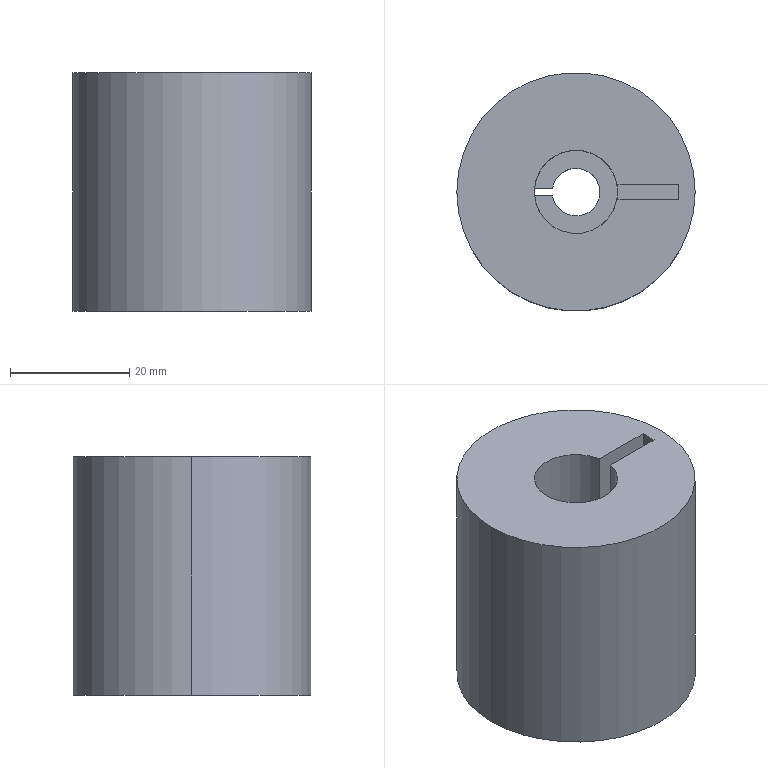Part | SolidWorks | features ICE 4, Extrusion 1 | 1 solid | 17 faces | box 40 x 40 x 40 mm | volume 44793 mm3 | plane 11 | cylinder 6 | commonest cylinder face diameters 8 x2 14 x2 40 x2
STEP:
#1=CARTESIAN_POINT('',(-7.,0.,13.));
#2=VERTEX_POINT('',#1);
#3=CARTESIAN_POINT('',(-6.971,-0.64,13.));
#4=VERTEX_POINT('',#3);
#5=CARTESIAN_POINT('',(0.,0.,13.));
#6=DIRECTION('',(0.,0.,1.));
#7=DIRECTION('',(-1.,0.,0.));
#8=AXIS2_PLACEMENT_3D('',#5,#6,#7);
#9=CIRCLE('',#8,7.);
#10=EDGE_CURVE('',#2,#4,#9,.T.);
#11=ORIENTED_EDGE('',*,*,#10,.F.);
#12=CARTESIAN_POINT('',(-7.,0.,40.));
#13=VERTEX_POINT('',#12);
#14=CARTESIAN_POINT('',(-7.,0.,12.));
#15=DIRECTION('',(0.,0.,1.));
#16=VECTOR('',#15,1000.);
#17=LINE('',#14,#16);
#18=EDGE_CURVE('',#2,#13,#17,.T.);
#19=ORIENTED_EDGE('',*,*,#18,.T.);
#20=CARTESIAN_POINT('',(6.878,-1.3,40.));
#21=VERTEX_POINT('',#20);
#22=CARTESIAN_POINT('',(0.,0.,40.));
#23=DIRECTION('',(0.,0.,1.));
#24=DIRECTION('',(1.,0.,0.));
#25=AXIS2_PLACEMENT_3D('',#22,#23,#24);
#26=CIRCLE('',#25,7.);
#27=EDGE_CURVE('',#13,#21,#26,.T.);
#28=ORIENTED_EDGE('',*,*,#27,.T.);
#29=CARTESIAN_POINT('',(6.878,-1.3,27.));
#30=VERTEX_POINT('',#29);
#31=CARTESIAN_POINT('',(6.878,-1.3,27.));
#32=DIRECTION('',(0.,0.,1.));
#33=VECTOR('',#32,1000.);
#34=LINE('',#31,#33);
#35=EDGE_CURVE('',#30,#21,#34,.T.);
#36=ORIENTED_EDGE('',*,*,#35,.F.);
#37=CARTESIAN_POINT('',(7.,0.,27.));
#38=VERTEX_POINT('',#37);
#39=CARTESIAN_POINT('',(0.,0.,27.));
#40=DIRECTION('',(0.,0.,-1.));
#41=DIRECTION('',(1.,0.,0.));
#42=AXIS2_PLACEMENT_3D('',#39,#40,#41);
#43=CIRCLE('',#42,7.);
#44=EDGE_CURVE('',#38,#30,#43,.T.);
#45=ORIENTED_EDGE('',*,*,#44,.F.);
#46=CARTESIAN_POINT('',(7.,0.,12.));
#47=VERTEX_POINT('',#46);
#48=CARTESIAN_POINT('',(7.,0.,12.));
#49=DIRECTION('',(0.,0.,1.));
#50=VECTOR('',#49,1000.);
#51=LINE('',#48,#50);
#52=EDGE_CURVE('',#47,#38,#51,.T.);
#53=ORIENTED_EDGE('',*,*,#52,.F.);
#54=CARTESIAN_POINT('',(-6.971,-0.64,12.));
#55=VERTEX_POINT('',#54);
#56=CARTESIAN_POINT('',(0.,0.,12.));
#57=DIRECTION('',(0.,0.,1.));
#58=DIRECTION('',(1.,0.,0.));
#59=AXIS2_PLACEMENT_3D('',#56,#57,#58);
#60=CIRCLE('',#59,7.);
#61=EDGE_CURVE('',#55,#47,#60,.T.);
#62=ORIENTED_EDGE('',*,*,#61,.F.);
#63=CARTESIAN_POINT('',(-6.971,-0.64,12.));
#64=DIRECTION('',(0.,0.,1.));
#65=VECTOR('',#64,1000.);
#66=LINE('',#63,#65);
#67=EDGE_CURVE('',#55,#4,#66,.T.);
#68=ORIENTED_EDGE('',*,*,#67,.T.);
#69=EDGE_LOOP('',(#11,#19,#28,#36,#45,#53,#62,#68));
#70=FACE_OUTER_BOUND('',#69,.T.);
#71=CARTESIAN_POINT('',(0.,0.,12.));
#72=DIRECTION('',(0.,0.,1.));
#73=DIRECTION('',(1.,0.,0.));
#74=AXIS2_PLACEMENT_3D('',#71,#72,#73);
#75=CYLINDRICAL_SURFACE('',#74,7.);
#76=ADVANCED_FACE('',(#70),#75,.F.);
#77=CARTESIAN_POINT('',(20.,0.,40.));
#78=VERTEX_POINT('',#77);
#79=CARTESIAN_POINT('',(-20.,0.,40.));
#80=VERTEX_POINT('',#79);
#81=CARTESIAN_POINT('',(0.,0.,40.));
#82=DIRECTION('',(0.,0.,1.));
#83=DIRECTION('',(1.,0.,0.));
#84=AXIS2_PLACEMENT_3D('',#81,#82,#83);
#85=CIRCLE('',#84,20.);
#86=EDGE_CURVE('',#78,#80,#85,.T.);
#87=ORIENTED_EDGE('',*,*,#86,.F.);
#88=CARTESIAN_POINT('',(20.,0.,0.));
#89=VERTEX_POINT('',#88);
#90=CARTESIAN_POINT('',(20.,0.,40.));
#91=DIRECTION('',(0.,0.,-1.));
#92=VECTOR('',#91,1000.);
#93=LINE('',#90,#92);
#94=EDGE_CURVE('',#78,#89,#93,.T.);
#95=ORIENTED_EDGE('',*,*,#94,.T.);
#96=CARTESIAN_POINT('',(-20.,0.,0.));
#97=VERTEX_POINT('',#96);
#98=CARTESIAN_POINT('',(0.,0.,0.));
#99=DIRECTION('',(0.,0.,1.));
#100=DIRECTION('',(1.,0.,0.));
#101=AXIS2_PLACEMENT_3D('',#98,#99,#100);
#102=CIRCLE('',#101,20.);
#103=EDGE_CURVE('',#89,#97,#102,.T.);
#104=ORIENTED_EDGE('',*,*,#103,.T.);
#105=CARTESIAN_POINT('',(-20.,0.,40.));
#106=DIRECTION('',(0.,0.,-1.));
#107=VECTOR('',#106,1000.);
#108=LINE('',#105,#107);
#109=EDGE_CURVE('',#80,#97,#108,.T.);
#110=ORIENTED_EDGE('',*,*,#109,.F.);
#111=EDGE_LOOP('',(#87,#95,#104,#110));
#112=FACE_OUTER_BOUND('',#111,.T.);
#113=CARTESIAN_POINT('',(0.,0.,40.));
#114=DIRECTION('',(0.,0.,-1.));
#115=DIRECTION('',(-1.,0.,0.));
#116=AXIS2_PLACEMENT_3D('',#113,#114,#115);
#117=CYLINDRICAL_SURFACE('',#116,20.);
#118=ADVANCED_FACE('',(#112),#117,.T.);
#119=CARTESIAN_POINT('',(4.,0.,0.));
#120=VERTEX_POINT('',#119);
#121=CARTESIAN_POINT('',(-3.948,0.64,0.));
#122=VERTEX_POINT('',#121);
#123=CARTESIAN_POINT('',(0.,0.,0.));
#124=DIRECTION('',(0.,0.,1.));
#125=DIRECTION('',(1.,0.,0.));
#126=AXIS2_PLACEMENT_3D('',#123,#124,#125);
#127=CIRCLE('',#126,4.);
#128=EDGE_CURVE('',#120,#122,#127,.T.);
#129=ORIENTED_EDGE('',*,*,#128,.F.);
#130=CARTESIAN_POINT('',(4.,0.,12.));
#131=VERTEX_POINT('',#130);
#132=CARTESIAN_POINT('',(4.,0.,0.));
#133=DIRECTION('',(0.,0.,1.));
#134=VECTOR('',#133,1000.);
#135=LINE('',#132,#134);
#136=EDGE_CURVE('',#120,#131,#135,.T.);
#137=ORIENTED_EDGE('',*,*,#136,.T.);
#138=CARTESIAN_POINT('',(-3.948,0.64,12.));
#139=VERTEX_POINT('',#138);
#140=CARTESIAN_POINT('',(0.,0.,12.));
#141=DIRECTION('',(0.,0.,-1.));
#142=DIRECTION('',(1.,0.,0.));
#143=AXIS2_PLACEMENT_3D('',#140,#141,#142);
#144=CIRCLE('',#143,4.);
#145=EDGE_CURVE('',#139,#131,#144,.T.);
#146=ORIENTED_EDGE('',*,*,#145,.F.);
#147=CARTESIAN_POINT('',(-3.948,0.64,13.));
#148=DIRECTION('',(0.,0.,-1.));
#149=VECTOR('',#148,1000.);
#150=LINE('',#147,#149);
#151=EDGE_CURVE('',#139,#122,#150,.T.);
#152=ORIENTED_EDGE('',*,*,#151,.T.);
#153=EDGE_LOOP('',(#129,#137,#146,#152));
#154=FACE_OUTER_BOUND('',#153,.T.);
#155=CARTESIAN_POINT('',(0.,0.,0.));
#156=DIRECTION('',(0.,0.,1.));
#157=DIRECTION('',(1.,0.,0.));
#158=AXIS2_PLACEMENT_3D('',#155,#156,#157);
#159=CYLINDRICAL_SURFACE('',#158,4.);
#160=ADVANCED_FACE('',(#154),#159,.F.);
#161=ORIENTED_EDGE('',*,*,#136,.F.);
#162=CARTESIAN_POINT('',(-3.948,-0.64,0.));
#163=VERTEX_POINT('',#162);
#164=CARTESIAN_POINT('',(0.,0.,0.));
#165=DIRECTION('',(0.,0.,1.));
#166=DIRECTION('',(1.,0.,0.));
#167=AXIS2_PLACEMENT_3D('',#164,#165,#166);
#168=CIRCLE('',#167,4.);
#169=EDGE_CURVE('',#163,#120,#168,.T.);
#170=ORIENTED_EDGE('',*,*,#169,.F.);
#171=CARTESIAN_POINT('',(-3.948,-0.64,12.));
#172=VERTEX_POINT('',#171);
#173=CARTESIAN_POINT('',(-3.948,-0.64,13.));
#174=DIRECTION('',(0.,0.,-1.));
#175=VECTOR('',#174,1000.);
#176=LINE('',#173,#175);
#177=EDGE_CURVE('',#172,#163,#176,.T.);
#178=ORIENTED_EDGE('',*,*,#177,.F.);
#179=CARTESIAN_POINT('',(0.,0.,12.));
#180=DIRECTION('',(0.,0.,-1.));
#181=DIRECTION('',(1.,0.,0.));
#182=AXIS2_PLACEMENT_3D('',#179,#180,#181);
#183=CIRCLE('',#182,4.);
#184=EDGE_CURVE('',#131,#172,#183,.T.);
#185=ORIENTED_EDGE('',*,*,#184,.F.);
#186=EDGE_LOOP('',(#161,#170,#178,#185));
#187=FACE_OUTER_BOUND('',#186,.T.);
#188=CARTESIAN_POINT('',(0.,0.,0.));
#189=DIRECTION('',(0.,0.,1.));
#190=DIRECTION('',(1.,0.,0.));
#191=AXIS2_PLACEMENT_3D('',#188,#189,#190);
#192=CYLINDRICAL_SURFACE('',#191,4.);
#193=ADVANCED_FACE('',(#187),#192,.F.);
#194=ORIENTED_EDGE('',*,*,#94,.F.);
#195=CARTESIAN_POINT('',(0.,0.,40.));
#196=DIRECTION('',(0.,0.,1.));
#197=DIRECTION('',(1.,0.,0.));
#198=AXIS2_PLACEMENT_3D('',#195,#196,#197);
#199=CIRCLE('',#198,20.);
#200=EDGE_CURVE('',#80,#78,#199,.T.);
#201=ORIENTED_EDGE('',*,*,#200,.F.);
#202=ORIENTED_EDGE('',*,*,#109,.T.);
#203=CARTESIAN_POINT('',(0.,0.,0.));
#204=DIRECTION('',(0.,0.,1.));
#205=DIRECTION('',(1.,0.,0.));
#206=AXIS2_PLACEMENT_3D('',#203,#204,#205);
#207=CIRCLE('',#206,20.);
#208=EDGE_CURVE('',#97,#89,#207,.T.);
#209=ORIENTED_EDGE('',*,*,#208,.T.);
#210=EDGE_LOOP('',(#194,#201,#202,#209));
#211=FACE_OUTER_BOUND('',#210,.T.);
#212=CARTESIAN_POINT('',(0.,0.,40.));
#213=DIRECTION('',(0.,0.,-1.));
#214=DIRECTION('',(-1.,0.,0.));
#215=AXIS2_PLACEMENT_3D('',#212,#213,#214);
#216=CYLINDRICAL_SURFACE('',#215,20.);
#217=ADVANCED_FACE('',(#211),#216,.T.);
#218=CARTESIAN_POINT('',(17.228,1.3,40.));
#219=VERTEX_POINT('',#218);
#220=CARTESIAN_POINT('',(6.878,1.3,40.));
#221=VERTEX_POINT('',#220);
#222=CARTESIAN_POINT('',(17.228,1.3,40.));
#223=DIRECTION('',(-1.,0.,0.));
#224=VECTOR('',#223,1000.);
#225=LINE('',#222,#224);
#226=EDGE_CURVE('',#219,#221,#225,.T.);
#227=ORIENTED_EDGE('',*,*,#226,.F.);
#228=CARTESIAN_POINT('',(17.228,-1.3,40.));
#229=VERTEX_POINT('',#228);
#230=CARTESIAN_POINT('',(17.228,-1.3,40.));
#231=DIRECTION('',(0.,1.,0.));
#232=VECTOR('',#231,1000.);
#233=LINE('',#230,#232);
#234=EDGE_CURVE('',#229,#219,#233,.T.);
#235=ORIENTED_EDGE('',*,*,#234,.F.);
#236=CARTESIAN_POINT('',(17.228,-1.3,40.));
#237=DIRECTION('',(1.,0.,0.));
#238=VECTOR('',#237,1000.);
#239=LINE('',#236,#238);
#240=EDGE_CURVE('',#21,#229,#239,.T.);
#241=ORIENTED_EDGE('',*,*,#240,.F.);
#242=ORIENTED_EDGE('',*,*,#27,.F.);
#243=CARTESIAN_POINT('',(0.,0.,40.));
#244=DIRECTION('',(0.,0.,1.));
#245=DIRECTION('',(1.,0.,0.));
#246=AXIS2_PLACEMENT_3D('',#243,#244,#245);
#247=CIRCLE('',#246,7.);
#248=EDGE_CURVE('',#221,#13,#247,.T.);
#249=ORIENTED_EDGE('',*,*,#248,.F.);
#250=EDGE_LOOP('',(#227,#235,#241,#242,#249));
#251=FACE_BOUND('',#250,.T.);
#252=ORIENTED_EDGE('',*,*,#200,.T.);
#253=ORIENTED_EDGE('',*,*,#86,.T.);
#254=EDGE_LOOP('',(#252,#253));
#255=FACE_OUTER_BOUND('',#254,.T.);
#256=CARTESIAN_POINT('',(0.,0.,40.));
#257=DIRECTION('',(0.,0.,1.));
#258=DIRECTION('',(1.,0.,0.));
#259=AXIS2_PLACEMENT_3D('',#256,#257,#258);
#260=PLANE('',#259);
#261=ADVANCED_FACE('',(#251,#255),#260,.T.);
#262=ORIENTED_EDGE('',*,*,#169,.T.);
#263=ORIENTED_EDGE('',*,*,#128,.T.);
#264=CARTESIAN_POINT('',(-16.948,0.64,0.));
#265=VERTEX_POINT('',#264);
#266=CARTESIAN_POINT('',(-16.948,0.64,0.));
#267=DIRECTION('',(1.,0.,0.));
#268=VECTOR('',#267,1000.);
#269=LINE('',#266,#268);
#270=EDGE_CURVE('',#265,#122,#269,.T.);
#271=ORIENTED_EDGE('',*,*,#270,.F.);
#272=CARTESIAN_POINT('',(-16.948,-0.64,0.));
#273=VERTEX_POINT('',#272);
#274=CARTESIAN_POINT('',(-16.948,-0.64,0.));
#275=DIRECTION('',(0.,1.,0.));
#276=VECTOR('',#275,1000.);
#277=LINE('',#274,#276);
#278=EDGE_CURVE('',#273,#265,#277,.T.);
#279=ORIENTED_EDGE('',*,*,#278,.F.);
#280=CARTESIAN_POINT('',(-16.948,-0.64,0.));
#281=DIRECTION('',(-1.,0.,0.));
#282=VECTOR('',#281,1000.);
#283=LINE('',#280,#282);
#284=EDGE_CURVE('',#163,#273,#283,.T.);
#285=ORIENTED_EDGE('',*,*,#284,.F.);
#286=EDGE_LOOP('',(#262,#263,#271,#279,#285));
#287=FACE_BOUND('',#286,.T.);
#288=ORIENTED_EDGE('',*,*,#208,.F.);
#289=ORIENTED_EDGE('',*,*,#103,.F.);
#290=EDGE_LOOP('',(#288,#289));
#291=FACE_OUTER_BOUND('',#290,.T.);
#292=CARTESIAN_POINT('',(0.,0.,0.));
#293=DIRECTION('',(0.,0.,1.));
#294=DIRECTION('',(1.,0.,0.));
#295=AXIS2_PLACEMENT_3D('',#292,#293,#294);
#296=PLANE('',#295);
#297=ADVANCED_FACE('',(#287,#291),#296,.F.);
#298=CARTESIAN_POINT('',(-6.971,0.64,12.));
#299=VERTEX_POINT('',#298);
#300=CARTESIAN_POINT('',(0.,0.64,12.));
#301=DIRECTION('',(-1.,0.,0.));
#302=VECTOR('',#301,1000.);
#303=LINE('',#300,#302);
#304=EDGE_CURVE('',#139,#299,#303,.T.);
#305=ORIENTED_EDGE('',*,*,#304,.F.);
#306=ORIENTED_EDGE('',*,*,#145,.T.);
#307=ORIENTED_EDGE('',*,*,#184,.T.);
#308=CARTESIAN_POINT('',(0.,-0.64,12.));
#309=DIRECTION('',(1.,0.,0.));
#310=VECTOR('',#309,1000.);
#311=LINE('',#308,#310);
#312=EDGE_CURVE('',#55,#172,#311,.T.);
#313=ORIENTED_EDGE('',*,*,#312,.F.);
#314=ORIENTED_EDGE('',*,*,#61,.T.);
#315=CARTESIAN_POINT('',(0.,0.,12.));
#316=DIRECTION('',(0.,0.,1.));
#317=DIRECTION('',(1.,0.,0.));
#318=AXIS2_PLACEMENT_3D('',#315,#316,#317);
#319=CIRCLE('',#318,7.);
#320=EDGE_CURVE('',#47,#299,#319,.T.);
#321=ORIENTED_EDGE('',*,*,#320,.T.);
#322=EDGE_LOOP('',(#305,#306,#307,#313,#314,#321));
#323=FACE_OUTER_BOUND('',#322,.T.);
#324=CARTESIAN_POINT('',(0.,0.,12.));
#325=DIRECTION('',(0.,0.,1.));
#326=DIRECTION('',(1.,0.,0.));
#327=AXIS2_PLACEMENT_3D('',#324,#325,#326);
#328=PLANE('',#327);
#329=ADVANCED_FACE('',(#323),#328,.T.);
#330=ORIENTED_EDGE('',*,*,#18,.F.);
#331=CARTESIAN_POINT('',(-6.971,0.64,13.));
#332=VERTEX_POINT('',#331);
#333=CARTESIAN_POINT('',(0.,0.,13.));
#334=DIRECTION('',(0.,0.,1.));
#335=DIRECTION('',(-1.,0.,0.));
#336=AXIS2_PLACEMENT_3D('',#333,#334,#335);
#337=CIRCLE('',#336,7.);
#338=EDGE_CURVE('',#332,#2,#337,.T.);
#339=ORIENTED_EDGE('',*,*,#338,.F.);
#340=CARTESIAN_POINT('',(-6.971,0.64,12.));
#341=DIRECTION('',(0.,0.,-1.));
#342=VECTOR('',#341,1000.);
#343=LINE('',#340,#342);
#344=EDGE_CURVE('',#332,#299,#343,.T.);
#345=ORIENTED_EDGE('',*,*,#344,.T.);
#346=ORIENTED_EDGE('',*,*,#320,.F.);
#347=ORIENTED_EDGE('',*,*,#52,.T.);
#348=CARTESIAN_POINT('',(6.878,1.3,27.));
#349=VERTEX_POINT('',#348);
#350=CARTESIAN_POINT('',(0.,0.,27.));
#351=DIRECTION('',(0.,0.,-1.));
#352=DIRECTION('',(1.,0.,0.));
#353=AXIS2_PLACEMENT_3D('',#350,#351,#352);
#354=CIRCLE('',#353,7.);
#355=EDGE_CURVE('',#349,#38,#354,.T.);
#356=ORIENTED_EDGE('',*,*,#355,.F.);
#357=CARTESIAN_POINT('',(6.878,1.3,27.));
#358=DIRECTION('',(0.,0.,1.));
#359=VECTOR('',#358,1000.);
#360=LINE('',#357,#359);
#361=EDGE_CURVE('',#349,#221,#360,.T.);
#362=ORIENTED_EDGE('',*,*,#361,.T.);
#363=ORIENTED_EDGE('',*,*,#248,.T.);
#364=EDGE_LOOP('',(#330,#339,#345,#346,#347,#356,#362,#363));
#365=FACE_OUTER_BOUND('',#364,.T.);
#366=CARTESIAN_POINT('',(0.,0.,12.));
#367=DIRECTION('',(0.,0.,1.));
#368=DIRECTION('',(1.,0.,0.));
#369=AXIS2_PLACEMENT_3D('',#366,#367,#368);
#370=CYLINDRICAL_SURFACE('',#369,7.);
#371=ADVANCED_FACE('',(#365),#370,.F.);
#372=ORIENTED_EDGE('',*,*,#226,.T.);
#373=ORIENTED_EDGE('',*,*,#361,.F.);
#374=CARTESIAN_POINT('',(17.228,1.3,27.));
#375=VERTEX_POINT('',#374);
#376=CARTESIAN_POINT('',(17.228,1.3,27.));
#377=DIRECTION('',(-1.,0.,0.));
#378=VECTOR('',#377,1000.);
#379=LINE('',#376,#378);
#380=EDGE_CURVE('',#375,#349,#379,.T.);
#381=ORIENTED_EDGE('',*,*,#380,.F.);
#382=CARTESIAN_POINT('',(17.228,1.3,27.));
#383=DIRECTION('',(0.,0.,1.));
#384=VECTOR('',#383,1000.);
#385=LINE('',#382,#384);
#386=EDGE_CURVE('',#375,#219,#385,.T.);
#387=ORIENTED_EDGE('',*,*,#386,.T.);
#388=EDGE_LOOP('',(#372,#373,#381,#387));
#389=FACE_OUTER_BOUND('',#388,.T.);
#390=CARTESIAN_POINT('',(17.228,1.3,27.));
#391=DIRECTION('',(0.,1.,0.));
#392=DIRECTION('',(-1.,0.,0.));
#393=AXIS2_PLACEMENT_3D('',#390,#391,#392);
#394=PLANE('',#393);
#395=ADVANCED_FACE('',(#389),#394,.F.);
#396=ORIENTED_EDGE('',*,*,#234,.T.);
#397=ORIENTED_EDGE('',*,*,#386,.F.);
#398=CARTESIAN_POINT('',(17.228,-1.3,27.));
#399=VERTEX_POINT('',#398);
#400=CARTESIAN_POINT('',(17.228,-1.3,27.));
#401=DIRECTION('',(0.,1.,0.));
#402=VECTOR('',#401,1000.);
#403=LINE('',#400,#402);
#404=EDGE_CURVE('',#399,#375,#403,.T.);
#405=ORIENTED_EDGE('',*,*,#404,.F.);
#406=CARTESIAN_POINT('',(17.228,-1.3,27.));
#407=DIRECTION('',(0.,0.,1.));
#408=VECTOR('',#407,1000.);
#409=LINE('',#406,#408);
#410=EDGE_CURVE('',#399,#229,#409,.T.);
#411=ORIENTED_EDGE('',*,*,#410,.T.);
#412=EDGE_LOOP('',(#396,#397,#405,#411));
#413=FACE_OUTER_BOUND('',#412,.T.);
#414=CARTESIAN_POINT('',(17.228,-1.3,27.));
#415=DIRECTION('',(1.,0.,0.));
#416=DIRECTION('',(0.,0.,-1.));
#417=AXIS2_PLACEMENT_3D('',#414,#415,#416);
#418=PLANE('',#417);
#419=ADVANCED_FACE('',(#413),#418,.F.);
#420=ORIENTED_EDGE('',*,*,#240,.T.);
#421=ORIENTED_EDGE('',*,*,#410,.F.);
#422=CARTESIAN_POINT('',(17.228,-1.3,27.));
#423=DIRECTION('',(1.,0.,0.));
#424=VECTOR('',#423,1000.);
#425=LINE('',#422,#424);
#426=EDGE_CURVE('',#30,#399,#425,.T.);
#427=ORIENTED_EDGE('',*,*,#426,.F.);
#428=ORIENTED_EDGE('',*,*,#35,.T.);
#429=EDGE_LOOP('',(#420,#421,#427,#428));
#430=FACE_OUTER_BOUND('',#429,.T.);
#431=CARTESIAN_POINT('',(17.228,-1.3,27.));
#432=DIRECTION('',(0.,-1.,0.));
#433=DIRECTION('',(1.,0.,0.));
#434=AXIS2_PLACEMENT_3D('',#431,#432,#433);
#435=PLANE('',#434);
#436=ADVANCED_FACE('',(#430),#435,.F.);
#437=ORIENTED_EDGE('',*,*,#355,.T.);
#438=ORIENTED_EDGE('',*,*,#44,.T.);
#439=ORIENTED_EDGE('',*,*,#426,.T.);
#440=ORIENTED_EDGE('',*,*,#404,.T.);
#441=ORIENTED_EDGE('',*,*,#380,.T.);
#442=EDGE_LOOP('',(#437,#438,#439,#440,#441));
#443=FACE_OUTER_BOUND('',#442,.T.);
#444=CARTESIAN_POINT('',(0.,0.,27.));
#445=DIRECTION('',(0.,0.,1.));
#446=DIRECTION('',(1.,0.,0.));
#447=AXIS2_PLACEMENT_3D('',#444,#445,#446);
#448=PLANE('',#447);
#449=ADVANCED_FACE('',(#443),#448,.T.);
#450=ORIENTED_EDGE('',*,*,#338,.T.);
#451=ORIENTED_EDGE('',*,*,#10,.T.);
#452=CARTESIAN_POINT('',(-16.948,-0.64,13.));
#453=VERTEX_POINT('',#452);
#454=CARTESIAN_POINT('',(-16.948,-0.64,13.));
#455=DIRECTION('',(-1.,0.,0.));
#456=VECTOR('',#455,1000.);
#457=LINE('',#454,#456);
#458=EDGE_CURVE('',#4,#453,#457,.T.);
#459=ORIENTED_EDGE('',*,*,#458,.T.);
#460=CARTESIAN_POINT('',(-16.948,0.64,13.));
#461=VERTEX_POINT('',#460);
#462=CARTESIAN_POINT('',(-16.948,-0.64,13.));
#463=DIRECTION('',(0.,1.,0.));
#464=VECTOR('',#463,1000.);
#465=LINE('',#462,#464);
#466=EDGE_CURVE('',#453,#461,#465,.T.);
#467=ORIENTED_EDGE('',*,*,#466,.T.);
#468=CARTESIAN_POINT('',(-16.948,0.64,13.));
#469=DIRECTION('',(1.,0.,0.));
#470=VECTOR('',#469,1000.);
#471=LINE('',#468,#470);
#472=EDGE_CURVE('',#461,#332,#471,.T.);
#473=ORIENTED_EDGE('',*,*,#472,.T.);
#474=EDGE_LOOP('',(#450,#451,#459,#467,#473));
#475=FACE_OUTER_BOUND('',#474,.T.);
#476=CARTESIAN_POINT('',(0.,0.,13.));
#477=DIRECTION('',(0.,0.,-1.));
#478=DIRECTION('',(-1.,0.,0.));
#479=AXIS2_PLACEMENT_3D('',#476,#477,#478);
#480=PLANE('',#479);
#481=ADVANCED_FACE('',(#475),#480,.T.);
#482=ORIENTED_EDGE('',*,*,#304,.T.);
#483=ORIENTED_EDGE('',*,*,#344,.F.);
#484=ORIENTED_EDGE('',*,*,#472,.F.);
#485=CARTESIAN_POINT('',(-16.948,0.64,13.));
#486=DIRECTION('',(0.,0.,-1.));
#487=VECTOR('',#486,1000.);
#488=LINE('',#485,#487);
#489=EDGE_CURVE('',#461,#265,#488,.T.);
#490=ORIENTED_EDGE('',*,*,#489,.T.);
#491=ORIENTED_EDGE('',*,*,#270,.T.);
#492=ORIENTED_EDGE('',*,*,#151,.F.);
#493=EDGE_LOOP('',(#482,#483,#484,#490,#491,#492));
#494=FACE_OUTER_BOUND('',#493,.T.);
#495=CARTESIAN_POINT('',(-16.948,0.64,13.));
#496=DIRECTION('',(0.,1.,0.));
#497=DIRECTION('',(-1.,0.,0.));
#498=AXIS2_PLACEMENT_3D('',#495,#496,#497);
#499=PLANE('',#498);
#500=ADVANCED_FACE('',(#494),#499,.F.);
#501=ORIENTED_EDGE('',*,*,#278,.T.);
#502=ORIENTED_EDGE('',*,*,#489,.F.);
#503=ORIENTED_EDGE('',*,*,#466,.F.);
#504=CARTESIAN_POINT('',(-16.948,-0.64,13.));
#505=DIRECTION('',(0.,0.,-1.));
#506=VECTOR('',#505,1000.);
#507=LINE('',#504,#506);
#508=EDGE_CURVE('',#453,#273,#507,.T.);
#509=ORIENTED_EDGE('',*,*,#508,.T.);
#510=EDGE_LOOP('',(#501,#502,#503,#509));
#511=FACE_OUTER_BOUND('',#510,.T.);
#512=CARTESIAN_POINT('',(-16.948,-0.64,13.));
#513=DIRECTION('',(-1.,0.,0.));
#514=DIRECTION('',(0.,0.,1.));
#515=AXIS2_PLACEMENT_3D('',#512,#513,#514);
#516=PLANE('',#515);
#517=ADVANCED_FACE('',(#511),#516,.F.);
#518=ORIENTED_EDGE('',*,*,#312,.T.);
#519=ORIENTED_EDGE('',*,*,#177,.T.);
#520=ORIENTED_EDGE('',*,*,#284,.T.);
#521=ORIENTED_EDGE('',*,*,#508,.F.);
#522=ORIENTED_EDGE('',*,*,#458,.F.);
#523=ORIENTED_EDGE('',*,*,#67,.F.);
#524=EDGE_LOOP('',(#518,#519,#520,#521,#522,#523));
#525=FACE_OUTER_BOUND('',#524,.T.);
#526=CARTESIAN_POINT('',(-16.948,-0.64,13.));
#527=DIRECTION('',(0.,-1.,0.));
#528=DIRECTION('',(1.,0.,0.));
#529=AXIS2_PLACEMENT_3D('',#526,#527,#528);
#530=PLANE('',#529);
#531=ADVANCED_FACE('',(#525),#530,.F.);
#532=CLOSED_SHELL('',(#76,#118,#160,#193,#217,#261,#297,#329,#371,#395,#419,#436,#449,#481,#500,#517,#531));
#533=MANIFOLD_SOLID_BREP('',#532);
#534=CARTESIAN_POINT('',(0.,0.,0.));
#535=DIRECTION('',(0.,0.,1.));
#536=DIRECTION('',(1.,0.,0.));
#537=AXIS2_PLACEMENT_3D('',#534,#535,#536);
#538=(LENGTH_UNIT()NAMED_UNIT(*)SI_UNIT(.MILLI.,.METRE.));
#539=UNCERTAINTY_MEASURE_WITH_UNIT(LENGTH_MEASURE(0.00001),#538,'','');
#540=(NAMED_UNIT(*)PLANE_ANGLE_UNIT()SI_UNIT($,.RADIAN.));
#541=(NAMED_UNIT(*)SI_UNIT($,.STERADIAN.)SOLID_ANGLE_UNIT());
#542=(GEOMETRIC_REPRESENTATION_CONTEXT(3)GLOBAL_UNCERTAINTY_ASSIGNED_CONTEXT((#539))GLOBAL_UNIT_ASSIGNED_CONTEXT((#538,#540,#541))REPRESENTATION_CONTEXT('',''));
#543=ADVANCED_BREP_SHAPE_REPRESENTATION('',(#533,#537),#542);